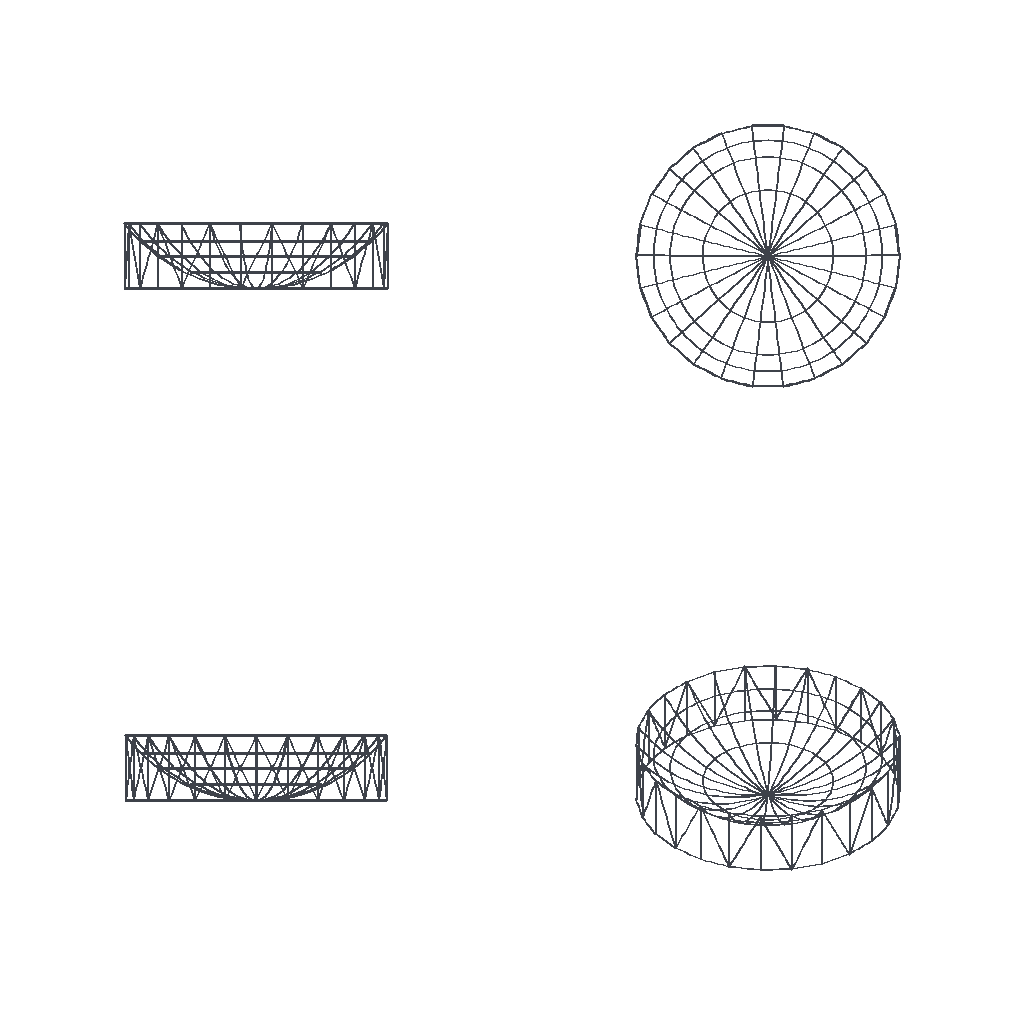Simulation study | abaqus
Set-up summary:
category,name,step,type,value,unit,region
solver,abaqus
solver,version,,,Abaqus/Standard 2020
units,not stated in the deck,,not stated
analysis,deck,,modal,modal
load_step,Step-1,Step-1,modal,nlgeom=False
contact,interactions,,,general=0 pairs=0 ties=0
load_step,requested,,,1
mesh,nodes,,,1578
mesh,elements,,,1681
element_type,B31,,beam,1681
load,load commands in deck,,count,0
bc,support commands in deck,,count,0
material,GAN,,in results
material,MATERIAL-3,,in results
material,QIAO,,in results
check,setup vs results,,match,"per instance, exact: element labels, types and connectivity; labels of the nodes the elements use; coordinates of those nodes at SINGLE_PRECISION in 1 of 1 instance(s)"
Abaqus input file, long lists of numbers shortened:
*Heading
** Job name: Job-5 Model name: Model-1-Copy-Copy
** Generated by: Abaqus/CAE 2020
*Preprint, echo=NO, model=NO, history=NO, contact=NO
**
** PARTS
**
*Part, name=ffff
*Node
      1,           0.,       -2000.,       -1500.
      2,  -482.147,  -3970.835,           0.
** (1576 more lines like these left out)
*Element, type=B31
 1,   1,  83
 2,  83,  84
** (1679 more lines like these left out)
*Nset, nset=Set-1
    2,    3,    4,    5,    6,    7,    8,    9,   10,   11,   12,   13,   14,   15,   16,   17
   18,   19,   20,   21,   22,   23,   24,   25,   26,   27,   28,   29,   30,   31,   32,   33
** (81 more lines like these left out)
*Elset, elset=Set-1
   64,   65,   66,   67,   68,   69,   70,   71,   72,   73,   74,   75,   76,   77,   78,   79
   80,   81,   82,   83,   84,   85,   86,   87,   88,   89,   90,   91,   92,   93,   94,   95
** (86 more lines like these left out)
*Nset, nset=Set-2
    1,   10,   12,   15,   16,   19,   20,   23,   24,   27,   28,   31,   32,   35,   36,   37
   38,   39,   43,   44,   45,   46,   51,   52,   54,   56,   62,   63,   82,   83,   84,   85
** (16 more lines like these left out)
*Elset, elset=Set-2
    1,    2,    3,    4,    5,    6,    7,    8,    9,   10,   11,   12,   13,   14,   15,   16
   17,   18,   19,   20,   21,   22,   23,   24,   25,   26,   27,   28,   29,   30,   31,   32
** (16 more lines like these left out)
*Nset, nset=Set-7, generate
    1,  1578,     1
*Elset, elset=Set-7, generate
    1,  1681,     1
*Nset, nset=Set-9, generate
    1,  1578,     1
*Elset, elset=Set-9, generate
    1,  1681,     1
*Nset, nset=Set-10, generate
    1,  1578,     1
*Elset, elset=Set-10, generate
    1,  1681,     1
** Section: Section-5  Profile: Profile-1
*Beam Section, elset=Set-9, material=gan, temperature=GRADIENTS, section=CIRC
50.
0.,1.,-1.
*End Part
**
**
** ASSEMBLY
**
*Assembly, name=Assembly
**
*Instance, name=ffff-1, part=ffff
*End Instance
**
*Nset, nset=Set-8, instance=ffff-1
    4,    5,    6,    8,   41,   49,   50,   53,   55,   57,   58,   60,   67,   68,   70,   71
   72,   73,   74,   75,   76,   77,   78,   79,   80,   81,  159,  160,  161,  162,  163,  164
** (7 more lines like these left out)
*Elset, elset=Set-8, instance=ffff-1
   80,   81,   82,   83,   84,   85,   86,   87,   88,   89,  111,  112,  113,  114,  115,  595
  596,  597,  598,  599, 1046, 1047, 1048, 1049, 1050, 1079, 1080, 1081, 1082, 1083, 1160, 1161
** (7 more lines like these left out)
*Nset, nset=m_Set-1, instance=ffff-1
  1,  2,  3,  7,  9, 13, 14, 17, 18, 21, 22, 25, 26, 29, 30, 33
 34, 40, 42, 45, 47, 48, 59, 61, 64, 65, 66, 69, 82
*Nset, nset=s_Set-5, instance=ffff-1
  2,  3,  7,  9, 13, 14, 17, 18, 21, 22, 25, 26, 30, 33, 34, 40
 42, 47, 48, 59, 61, 64, 65, 66, 69
*Nset, nset=s_Set-6, instance=ffff-1
  2,  3,  7,  9, 13, 14, 17, 18, 21, 22, 25, 26, 29, 30, 33, 34
 40, 42, 47, 48, 59, 61, 64, 65, 66, 69
*Nset, nset=s_Set-7, instance=ffff-1
    1,    2,    3,    7,    9,   10,   12,   13,   14,   15,   16,   17,   18,   19,   20,   21
   22,   23,   24,   25,   26,   27,   28,   29,   30,   31,   32,   33,   34,   35,   36,   37
** (26 more lines like these left out)
*Elset, elset=s_Set-7, instance=ffff-1
    1,    2,    3,    4,    5,    6,    7,    8,    9,   10,   11,   12,   13,   14,   15,   16
   17,   18,   19,   20,   21,   22,   23,   24,   25,   26,   27,   28,   29,   30,   31,   32
** (28 more lines like these left out)
*Nset, nset=s_Set-9, instance=ffff-1
    1,    2,    3,    7,    9,   10,   12,   13,   14,   15,   16,   17,   18,   19,   20,   21
   22,   23,   24,   25,   26,   27,   28,   29,   30,   31,   32,   33,   34,   35,   36,   37
** (26 more lines like these left out)
*Elset, elset=s_Set-9, instance=ffff-1
    1,    2,    3,    4,    5,    6,    7,    8,    9,   10,   11,   12,   13,   14,   15,   16
   17,   18,   19,   20,   21,   22,   23,   24,   25,   26,   27,   28,   29,   30,   31,   32
** (28 more lines like these left out)
*End Assembly
**
** MATERIALS
**
*Material, name=Material-3
*Density
 2.84e-09,
*Elastic
70000., 0.3
*Material, name=gan
*Density
 1.45e-09,
*Elastic
124000., 0.3
*Material, name=qiao
*Density
 4.5e-10,
*Elastic
10., 0.3
** ----------------------------------------------------------------
**
** STEP: Step-1
**
*Step, name=Step-1, nlgeom=NO, perturbation
*Frequency, eigensolver=Lanczos, sim, acoustic coupling=on, normalization=mass
5, , , , ,
**
** OUTPUT REQUESTS
**
*Restart, write, frequency=0
**
** FIELD OUTPUT: F-Output-1
**
*Output, field, variable=PRESELECT
*End Step
Results summary:
result,step,,partial,increments=0 time=0.0/1e-36
result,analysis,,,modal
result,last_loadstep,,,1
result,analysis steps,,count,1
result,primary field,,,"U, UR"